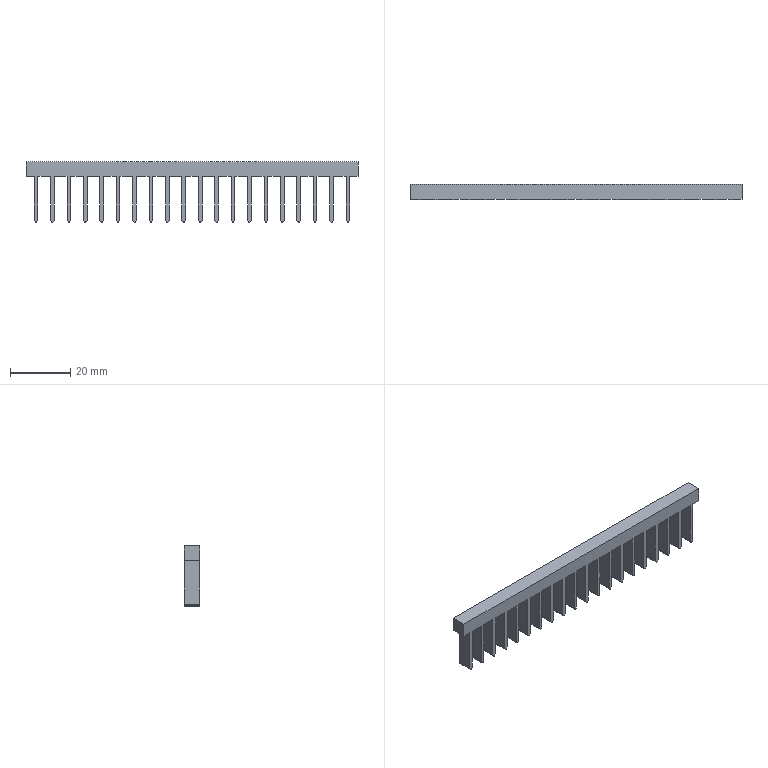Part | STEP file | 1 solid | 126 faces | box 110 x 4.97 x 20 mm | volume 4432 mm3 | plane 106 | cylinder 20 | commonest cylinder face diameters 0.68 x20